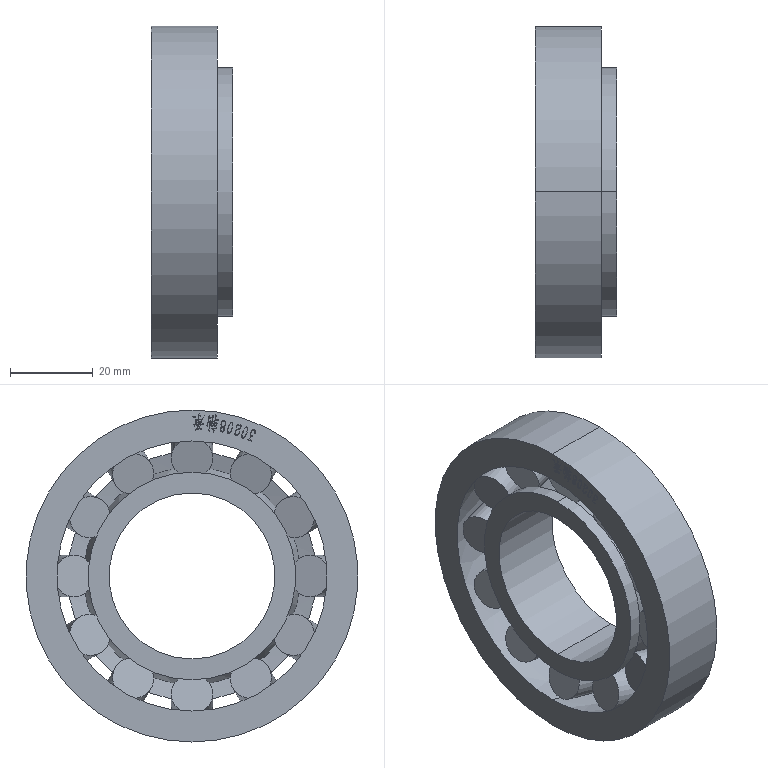Part | SolidWorks | features Revolution 5, CirPattern 1, ICE 1 | 17 solids | 454 faces | box 19.75 x 80 x 80 mm | volume 48755 mm3 | plane 280 | spline 128 | cylinder 38 | cone 8 | commonest cylinder face diameters 10 x30 40 x2 50 x2 60 x2 80 x2